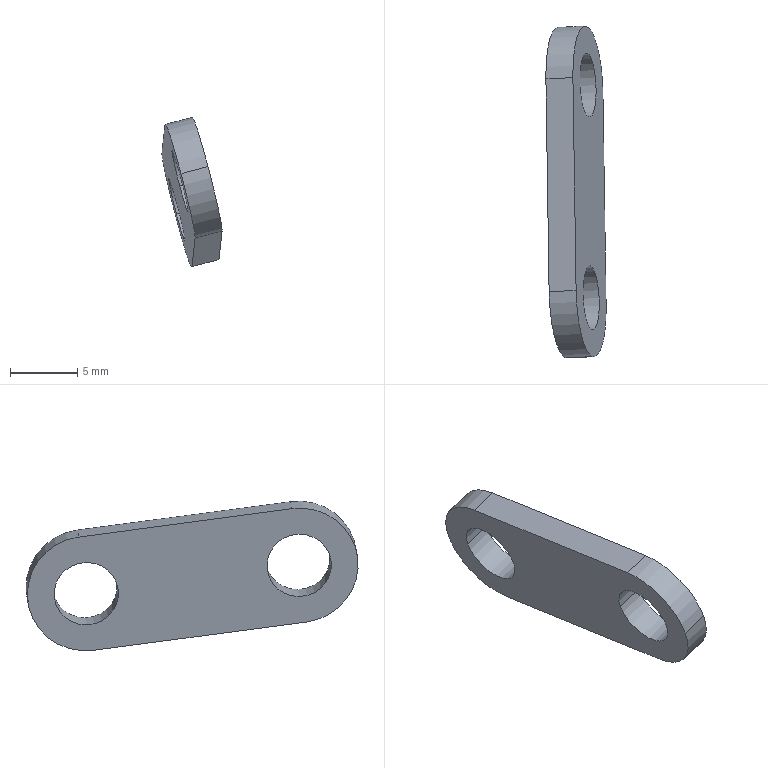Part | SolidWorks | features SplitBody 1 | 1 solid | 11 faces | box 4.488 x 24.748 x 11.149 mm | volume 344.095 mm3 | cylinder 7 | plane 4 | commonest cylinder face diameters 4.8 x4 8.8 x3
STEP:
#1=CARTESIAN_POINT('',(548.76,305.362,-381.709));
#2=VERTEX_POINT('',#1);
#3=CARTESIAN_POINT('',(548.689,310.119,-382.341));
#4=VERTEX_POINT('',#3);
#5=CARTESIAN_POINT('',(548.724,307.741,-382.025));
#6=DIRECTION('',(0.9671,0.04774,0.2498));
#7=DIRECTION('',(-0.01489,0.9912,-0.1318));
#8=AXIS2_PLACEMENT_3D('',#5,#6,#7);
#9=CIRCLE('',#8,2.4);
#10=EDGE_CURVE('',#2,#4,#9,.T.);
#11=ORIENTED_EDGE('',*,*,#10,.T.);
#12=CARTESIAN_POINT('',(546.677,310.02,-382.861));
#13=VERTEX_POINT('',#12);
#14=CARTESIAN_POINT('',(548.689,310.119,-382.341));
#15=DIRECTION('',(-0.9671,-0.04774,-0.2498));
#16=VECTOR('',#15,1000.);
#17=LINE('',#14,#16);
#18=EDGE_CURVE('',#4,#13,#17,.T.);
#19=ORIENTED_EDGE('',*,*,#18,.T.);
#20=CARTESIAN_POINT('',(546.748,305.262,-382.228));
#21=VERTEX_POINT('',#20);
#22=CARTESIAN_POINT('',(546.713,307.641,-382.544));
#23=DIRECTION('',(0.9671,0.04774,0.2498));
#24=DIRECTION('',(-0.01489,0.9912,-0.1318));
#25=AXIS2_PLACEMENT_3D('',#22,#23,#24);
#26=CIRCLE('',#25,2.4);
#27=EDGE_CURVE('',#21,#13,#26,.T.);
#28=ORIENTED_EDGE('',*,*,#27,.F.);
#29=CARTESIAN_POINT('',(548.76,305.362,-381.709));
#30=DIRECTION('',(-0.9671,-0.04774,-0.2498));
#31=VECTOR('',#30,1000.);
#32=LINE('',#29,#31);
#33=EDGE_CURVE('',#2,#21,#32,.T.);
#34=ORIENTED_EDGE('',*,*,#33,.F.);
#35=EDGE_LOOP('',(#11,#19,#28,#34));
#36=FACE_OUTER_BOUND('',#35,.T.);
#37=CARTESIAN_POINT('',(548.724,307.741,-382.025));
#38=DIRECTION('',(-0.9671,-0.04774,-0.2498));
#39=DIRECTION('',(0.01489,-0.9912,0.1318));
#40=AXIS2_PLACEMENT_3D('',#37,#38,#39);
#41=CYLINDRICAL_SURFACE('',#40,2.4);
#42=ADVANCED_FACE('',(#36),#41,.F.);
#43=CARTESIAN_POINT('',(548.998,289.503,-379.6));
#44=VERTEX_POINT('',#43);
#45=CARTESIAN_POINT('',(548.927,294.261,-380.233));
#46=VERTEX_POINT('',#45);
#47=CARTESIAN_POINT('',(548.963,291.882,-379.916));
#48=DIRECTION('',(0.9671,0.04774,0.2498));
#49=DIRECTION('',(-0.01489,0.9912,-0.1318));
#50=AXIS2_PLACEMENT_3D('',#47,#48,#49);
#51=CIRCLE('',#50,2.4);
#52=EDGE_CURVE('',#44,#46,#51,.T.);
#53=ORIENTED_EDGE('',*,*,#52,.T.);
#54=CARTESIAN_POINT('',(546.915,294.161,-380.752));
#55=VERTEX_POINT('',#54);
#56=CARTESIAN_POINT('',(548.927,294.261,-380.233));
#57=DIRECTION('',(-0.9671,-0.04774,-0.2498));
#58=VECTOR('',#57,1000.);
#59=LINE('',#56,#58);
#60=EDGE_CURVE('',#46,#55,#59,.T.);
#61=ORIENTED_EDGE('',*,*,#60,.T.);
#62=CARTESIAN_POINT('',(546.987,289.404,-380.12));
#63=VERTEX_POINT('',#62);
#64=CARTESIAN_POINT('',(546.951,291.783,-380.436));
#65=DIRECTION('',(0.9671,0.04774,0.2498));
#66=DIRECTION('',(-0.01489,0.9912,-0.1318));
#67=AXIS2_PLACEMENT_3D('',#64,#65,#66);
#68=CIRCLE('',#67,2.4);
#69=EDGE_CURVE('',#63,#55,#68,.T.);
#70=ORIENTED_EDGE('',*,*,#69,.F.);
#71=CARTESIAN_POINT('',(548.998,289.503,-379.6));
#72=DIRECTION('',(-0.9671,-0.04774,-0.2498));
#73=VECTOR('',#72,1000.);
#74=LINE('',#71,#73);
#75=EDGE_CURVE('',#44,#63,#74,.T.);
#76=ORIENTED_EDGE('',*,*,#75,.F.);
#77=EDGE_LOOP('',(#53,#61,#70,#76));
#78=FACE_OUTER_BOUND('',#77,.T.);
#79=CARTESIAN_POINT('',(548.963,291.882,-379.916));
#80=DIRECTION('',(-0.9671,-0.04774,-0.2498));
#81=DIRECTION('',(0.01489,-0.9912,0.1318));
#82=AXIS2_PLACEMENT_3D('',#79,#80,#81);
#83=CYLINDRICAL_SURFACE('',#82,2.4);
#84=ADVANCED_FACE('',(#78),#83,.F.);
#85=CARTESIAN_POINT('',(549.028,287.521,-379.337));
#86=VERTEX_POINT('',#85);
#87=CARTESIAN_POINT('',(550.08,291.338,-384.137));
#88=VERTEX_POINT('',#87);
#89=CARTESIAN_POINT('',(548.963,291.882,-379.916));
#90=DIRECTION('',(0.9671,0.04774,0.2498));
#91=DIRECTION('',(0.01489,-0.9912,0.1318));
#92=AXIS2_PLACEMENT_3D('',#89,#90,#91);
#93=CIRCLE('',#92,4.4);
#94=EDGE_CURVE('',#86,#88,#93,.T.);
#95=ORIENTED_EDGE('',*,*,#94,.F.);
#96=CARTESIAN_POINT('',(547.016,287.421,-379.856));
#97=VERTEX_POINT('',#96);
#98=CARTESIAN_POINT('',(549.028,287.521,-379.337));
#99=DIRECTION('',(-0.9671,-0.04774,-0.2498));
#100=VECTOR('',#99,1000.);
#101=LINE('',#98,#100);
#102=EDGE_CURVE('',#86,#97,#101,.T.);
#103=ORIENTED_EDGE('',*,*,#102,.T.);
#104=CARTESIAN_POINT('',(548.068,291.238,-384.657));
#105=VERTEX_POINT('',#104);
#106=CARTESIAN_POINT('',(546.951,291.783,-380.436));
#107=DIRECTION('',(0.9671,0.04774,0.2498));
#108=DIRECTION('',(0.01489,-0.9912,0.1318));
#109=AXIS2_PLACEMENT_3D('',#106,#107,#108);
#110=CIRCLE('',#109,4.4);
#111=EDGE_CURVE('',#97,#105,#110,.T.);
#112=ORIENTED_EDGE('',*,*,#111,.T.);
#113=CARTESIAN_POINT('',(550.08,291.338,-384.137));
#114=DIRECTION('',(-0.9671,-0.04774,-0.2498));
#115=VECTOR('',#114,1000.);
#116=LINE('',#113,#115);
#117=EDGE_CURVE('',#88,#105,#116,.T.);
#118=ORIENTED_EDGE('',*,*,#117,.F.);
#119=EDGE_LOOP('',(#95,#103,#112,#118));
#120=FACE_OUTER_BOUND('',#119,.T.);
#121=CARTESIAN_POINT('',(548.963,291.882,-379.916));
#122=DIRECTION('',(-0.9671,-0.04774,-0.2498));
#123=DIRECTION('',(0.01489,-0.9912,0.1318));
#124=AXIS2_PLACEMENT_3D('',#121,#122,#123);
#125=CYLINDRICAL_SURFACE('',#124,4.4);
#126=ADVANCED_FACE('',(#120),#125,.T.);
#127=CARTESIAN_POINT('',(547.845,292.426,-375.696));
#128=VERTEX_POINT('',#127);
#129=CARTESIAN_POINT('',(548.963,291.882,-379.916));
#130=DIRECTION('',(0.9671,0.04774,0.2498));
#131=DIRECTION('',(0.01489,-0.9912,0.1318));
#132=AXIS2_PLACEMENT_3D('',#129,#130,#131);
#133=CIRCLE('',#132,4.4);
#134=EDGE_CURVE('',#128,#86,#133,.T.);
#135=ORIENTED_EDGE('',*,*,#134,.T.);
#136=ORIENTED_EDGE('',*,*,#94,.T.);
#137=CARTESIAN_POINT('',(549.841,307.196,-386.246));
#138=VERTEX_POINT('',#137);
#139=CARTESIAN_POINT('',(550.08,291.338,-384.137));
#140=DIRECTION('',(-0.01489,0.9912,-0.1318));
#141=VECTOR('',#140,1000.);
#142=LINE('',#139,#141);
#143=EDGE_CURVE('',#88,#138,#142,.T.);
#144=ORIENTED_EDGE('',*,*,#143,.T.);
#145=CARTESIAN_POINT('',(547.607,308.285,-377.804));
#146=VERTEX_POINT('',#145);
#147=CARTESIAN_POINT('',(548.724,307.741,-382.025));
#148=DIRECTION('',(0.9671,0.04774,0.2498));
#149=DIRECTION('',(-0.01489,0.9912,-0.1318));
#150=AXIS2_PLACEMENT_3D('',#147,#148,#149);
#151=CIRCLE('',#150,4.4);
#152=EDGE_CURVE('',#138,#146,#151,.T.);
#153=ORIENTED_EDGE('',*,*,#152,.T.);
#154=CARTESIAN_POINT('',(547.607,308.285,-377.804));
#155=DIRECTION('',(0.01489,-0.9912,0.1318));
#156=VECTOR('',#155,1000.);
#157=LINE('',#154,#156);
#158=EDGE_CURVE('',#146,#128,#157,.T.);
#159=ORIENTED_EDGE('',*,*,#158,.T.);
#160=EDGE_LOOP('',(#135,#136,#144,#153,#159));
#161=FACE_OUTER_BOUND('',#160,.T.);
#162=ORIENTED_EDGE('',*,*,#52,.F.);
#163=CARTESIAN_POINT('',(548.963,291.882,-379.916));
#164=DIRECTION('',(0.9671,0.04774,0.2498));
#165=DIRECTION('',(-0.01489,0.9912,-0.1318));
#166=AXIS2_PLACEMENT_3D('',#163,#164,#165);
#167=CIRCLE('',#166,2.4);
#168=EDGE_CURVE('',#46,#44,#167,.T.);
#169=ORIENTED_EDGE('',*,*,#168,.F.);
#170=EDGE_LOOP('',(#162,#169));
#171=FACE_BOUND('',#170,.T.);
#172=ORIENTED_EDGE('',*,*,#10,.F.);
#173=CARTESIAN_POINT('',(548.724,307.741,-382.025));
#174=DIRECTION('',(0.9671,0.04774,0.2498));
#175=DIRECTION('',(-0.01489,0.9912,-0.1318));
#176=AXIS2_PLACEMENT_3D('',#173,#174,#175);
#177=CIRCLE('',#176,2.4);
#178=EDGE_CURVE('',#4,#2,#177,.T.);
#179=ORIENTED_EDGE('',*,*,#178,.F.);
#180=EDGE_LOOP('',(#172,#179));
#181=FACE_BOUND('',#180,.T.);
#182=CARTESIAN_POINT('',(548.963,291.882,-379.916));
#183=DIRECTION('',(-0.9671,-0.04774,-0.2498));
#184=DIRECTION('',(0.01489,-0.9912,0.1318));
#185=AXIS2_PLACEMENT_3D('',#182,#183,#184);
#186=PLANE('',#185);
#187=ADVANCED_FACE('',(#161,#171,#181),#186,.F.);
#188=ORIENTED_EDGE('',*,*,#69,.T.);
#189=CARTESIAN_POINT('',(546.951,291.783,-380.436));
#190=DIRECTION('',(0.9671,0.04774,0.2498));
#191=DIRECTION('',(-0.01489,0.9912,-0.1318));
#192=AXIS2_PLACEMENT_3D('',#189,#190,#191);
#193=CIRCLE('',#192,2.4);
#194=EDGE_CURVE('',#55,#63,#193,.T.);
#195=ORIENTED_EDGE('',*,*,#194,.T.);
#196=EDGE_LOOP('',(#188,#195));
#197=FACE_BOUND('',#196,.T.);
#198=CARTESIAN_POINT('',(545.834,292.327,-376.215));
#199=VERTEX_POINT('',#198);
#200=CARTESIAN_POINT('',(546.951,291.783,-380.436));
#201=DIRECTION('',(0.9671,0.04774,0.2498));
#202=DIRECTION('',(0.01489,-0.9912,0.1318));
#203=AXIS2_PLACEMENT_3D('',#200,#201,#202);
#204=CIRCLE('',#203,4.4);
#205=EDGE_CURVE('',#199,#97,#204,.T.);
#206=ORIENTED_EDGE('',*,*,#205,.F.);
#207=CARTESIAN_POINT('',(545.596,308.186,-378.323));
#208=VERTEX_POINT('',#207);
#209=CARTESIAN_POINT('',(545.596,308.186,-378.323));
#210=DIRECTION('',(0.01489,-0.9912,0.1318));
#211=VECTOR('',#210,1000.);
#212=LINE('',#209,#211);
#213=EDGE_CURVE('',#208,#199,#212,.T.);
#214=ORIENTED_EDGE('',*,*,#213,.F.);
#215=CARTESIAN_POINT('',(547.83,307.097,-386.765));
#216=VERTEX_POINT('',#215);
#217=CARTESIAN_POINT('',(546.713,307.641,-382.544));
#218=DIRECTION('',(0.9671,0.04774,0.2498));
#219=DIRECTION('',(-0.01489,0.9912,-0.1318));
#220=AXIS2_PLACEMENT_3D('',#217,#218,#219);
#221=CIRCLE('',#220,4.4);
#222=EDGE_CURVE('',#216,#208,#221,.T.);
#223=ORIENTED_EDGE('',*,*,#222,.F.);
#224=CARTESIAN_POINT('',(548.068,291.238,-384.657));
#225=DIRECTION('',(-0.01489,0.9912,-0.1318));
#226=VECTOR('',#225,1000.);
#227=LINE('',#224,#226);
#228=EDGE_CURVE('',#105,#216,#227,.T.);
#229=ORIENTED_EDGE('',*,*,#228,.F.);
#230=ORIENTED_EDGE('',*,*,#111,.F.);
#231=EDGE_LOOP('',(#206,#214,#223,#229,#230));
#232=FACE_OUTER_BOUND('',#231,.T.);
#233=ORIENTED_EDGE('',*,*,#27,.T.);
#234=CARTESIAN_POINT('',(546.713,307.641,-382.544));
#235=DIRECTION('',(0.9671,0.04774,0.2498));
#236=DIRECTION('',(-0.01489,0.9912,-0.1318));
#237=AXIS2_PLACEMENT_3D('',#234,#235,#236);
#238=CIRCLE('',#237,2.4);
#239=EDGE_CURVE('',#13,#21,#238,.T.);
#240=ORIENTED_EDGE('',*,*,#239,.T.);
#241=EDGE_LOOP('',(#233,#240));
#242=FACE_BOUND('',#241,.T.);
#243=CARTESIAN_POINT('',(546.951,291.783,-380.436));
#244=DIRECTION('',(-0.9671,-0.04774,-0.2498));
#245=DIRECTION('',(0.01489,-0.9912,0.1318));
#246=AXIS2_PLACEMENT_3D('',#243,#244,#245);
#247=PLANE('',#246);
#248=ADVANCED_FACE('',(#197,#232,#242),#247,.T.);
#249=ORIENTED_EDGE('',*,*,#102,.F.);
#250=ORIENTED_EDGE('',*,*,#134,.F.);
#251=CARTESIAN_POINT('',(547.845,292.426,-375.696));
#252=DIRECTION('',(-0.9671,-0.04774,-0.2498));
#253=VECTOR('',#252,1000.);
#254=LINE('',#251,#253);
#255=EDGE_CURVE('',#128,#199,#254,.T.);
#256=ORIENTED_EDGE('',*,*,#255,.T.);
#257=ORIENTED_EDGE('',*,*,#205,.T.);
#258=EDGE_LOOP('',(#249,#250,#256,#257));
#259=FACE_OUTER_BOUND('',#258,.T.);
#260=CARTESIAN_POINT('',(548.963,291.882,-379.916));
#261=DIRECTION('',(-0.9671,-0.04774,-0.2498));
#262=DIRECTION('',(0.01489,-0.9912,0.1318));
#263=AXIS2_PLACEMENT_3D('',#260,#261,#262);
#264=CYLINDRICAL_SURFACE('',#263,4.4);
#265=ADVANCED_FACE('',(#259),#264,.T.);
#266=ORIENTED_EDGE('',*,*,#228,.T.);
#267=CARTESIAN_POINT('',(549.841,307.196,-386.246));
#268=DIRECTION('',(-0.9671,-0.04774,-0.2498));
#269=VECTOR('',#268,1000.);
#270=LINE('',#267,#269);
#271=EDGE_CURVE('',#138,#216,#270,.T.);
#272=ORIENTED_EDGE('',*,*,#271,.F.);
#273=ORIENTED_EDGE('',*,*,#143,.F.);
#274=ORIENTED_EDGE('',*,*,#117,.T.);
#275=EDGE_LOOP('',(#266,#272,#273,#274));
#276=FACE_OUTER_BOUND('',#275,.T.);
#277=CARTESIAN_POINT('',(550.08,291.338,-384.137));
#278=DIRECTION('',(-0.2539,0.1237,0.9593));
#279=DIRECTION('',(0.01489,-0.9912,0.1318));
#280=AXIS2_PLACEMENT_3D('',#277,#278,#279);
#281=PLANE('',#280);
#282=ADVANCED_FACE('',(#276),#281,.F.);
#283=ORIENTED_EDGE('',*,*,#222,.T.);
#284=CARTESIAN_POINT('',(547.607,308.285,-377.804));
#285=DIRECTION('',(-0.9671,-0.04774,-0.2498));
#286=VECTOR('',#285,1000.);
#287=LINE('',#284,#286);
#288=EDGE_CURVE('',#146,#208,#287,.T.);
#289=ORIENTED_EDGE('',*,*,#288,.F.);
#290=ORIENTED_EDGE('',*,*,#152,.F.);
#291=ORIENTED_EDGE('',*,*,#271,.T.);
#292=EDGE_LOOP('',(#283,#289,#290,#291));
#293=FACE_OUTER_BOUND('',#292,.T.);
#294=CARTESIAN_POINT('',(548.724,307.741,-382.025));
#295=DIRECTION('',(-0.9671,-0.04774,-0.2498));
#296=DIRECTION('',(0.01489,-0.9912,0.1318));
#297=AXIS2_PLACEMENT_3D('',#294,#295,#296);
#298=CYLINDRICAL_SURFACE('',#297,4.4);
#299=ADVANCED_FACE('',(#293),#298,.T.);
#300=ORIENTED_EDGE('',*,*,#213,.T.);
#301=ORIENTED_EDGE('',*,*,#255,.F.);
#302=ORIENTED_EDGE('',*,*,#158,.F.);
#303=ORIENTED_EDGE('',*,*,#288,.T.);
#304=EDGE_LOOP('',(#300,#301,#302,#303));
#305=FACE_OUTER_BOUND('',#304,.T.);
#306=CARTESIAN_POINT('',(547.607,308.285,-377.804));
#307=DIRECTION('',(0.2539,-0.1237,-0.9593));
#308=DIRECTION('',(-0.01489,0.9912,-0.1318));
#309=AXIS2_PLACEMENT_3D('',#306,#307,#308);
#310=PLANE('',#309);
#311=ADVANCED_FACE('',(#305),#310,.F.);
#312=ORIENTED_EDGE('',*,*,#60,.F.);
#313=ORIENTED_EDGE('',*,*,#168,.T.);
#314=ORIENTED_EDGE('',*,*,#75,.T.);
#315=ORIENTED_EDGE('',*,*,#194,.F.);
#316=EDGE_LOOP('',(#312,#313,#314,#315));
#317=FACE_OUTER_BOUND('',#316,.T.);
#318=CARTESIAN_POINT('',(548.963,291.882,-379.916));
#319=DIRECTION('',(-0.9671,-0.04774,-0.2498));
#320=DIRECTION('',(0.01489,-0.9912,0.1318));
#321=AXIS2_PLACEMENT_3D('',#318,#319,#320);
#322=CYLINDRICAL_SURFACE('',#321,2.4);
#323=ADVANCED_FACE('',(#317),#322,.F.);
#324=ORIENTED_EDGE('',*,*,#18,.F.);
#325=ORIENTED_EDGE('',*,*,#178,.T.);
#326=ORIENTED_EDGE('',*,*,#33,.T.);
#327=ORIENTED_EDGE('',*,*,#239,.F.);
#328=EDGE_LOOP('',(#324,#325,#326,#327));
#329=FACE_OUTER_BOUND('',#328,.T.);
#330=CARTESIAN_POINT('',(548.724,307.741,-382.025));
#331=DIRECTION('',(-0.9671,-0.04774,-0.2498));
#332=DIRECTION('',(0.01489,-0.9912,0.1318));
#333=AXIS2_PLACEMENT_3D('',#330,#331,#332);
#334=CYLINDRICAL_SURFACE('',#333,2.4);
#335=ADVANCED_FACE('',(#329),#334,.F.);
#336=CLOSED_SHELL('',(#42,#84,#126,#187,#248,#265,#282,#299,#311,#323,#335));
#337=MANIFOLD_SOLID_BREP('',#336);
#338=CARTESIAN_POINT('',(0.,0.,0.));
#339=DIRECTION('',(0.,0.,1.));
#340=DIRECTION('',(1.,0.,0.));
#341=AXIS2_PLACEMENT_3D('',#338,#339,#340);
#342=(LENGTH_UNIT()NAMED_UNIT(*)SI_UNIT(.MILLI.,.METRE.));
#343=UNCERTAINTY_MEASURE_WITH_UNIT(LENGTH_MEASURE(0.00001),#342,'','');
#344=(NAMED_UNIT(*)PLANE_ANGLE_UNIT()SI_UNIT($,.RADIAN.));
#345=(NAMED_UNIT(*)SI_UNIT($,.STERADIAN.)SOLID_ANGLE_UNIT());
#346=(GEOMETRIC_REPRESENTATION_CONTEXT(3)GLOBAL_UNCERTAINTY_ASSIGNED_CONTEXT((#343))GLOBAL_UNIT_ASSIGNED_CONTEXT((#342,#344,#345))REPRESENTATION_CONTEXT('',''));
#347=ADVANCED_BREP_SHAPE_REPRESENTATION('',(#337,#341),#346);